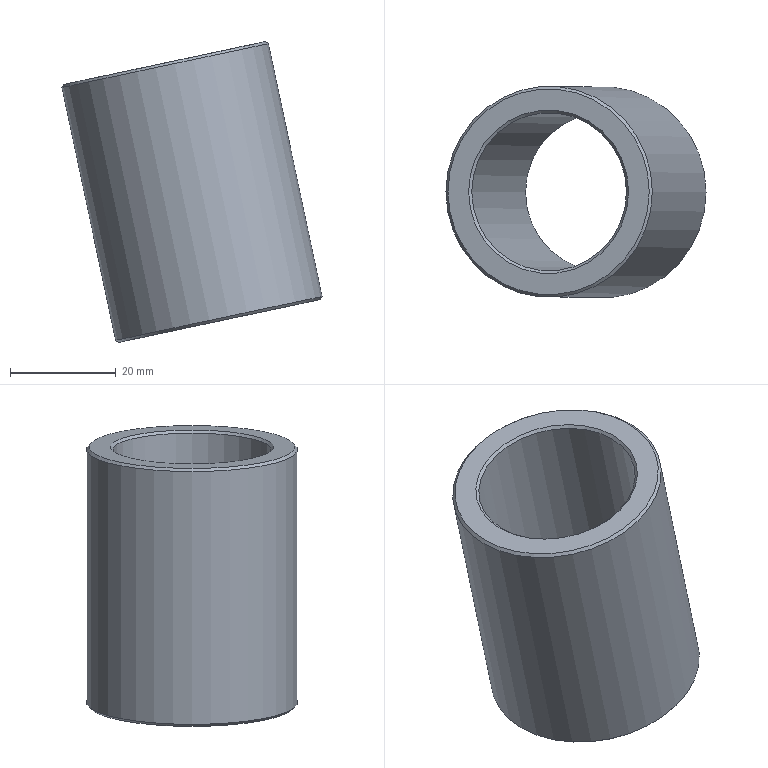Part | STEP file | solid 64 | 1 solid | 8 faces | box 49.314 x 40 x 57.016 mm | volume 27434 mm3 | cone 4 | plane 2 | cylinder 2 | commonest cylinder face diameters 30 x1 40 x1